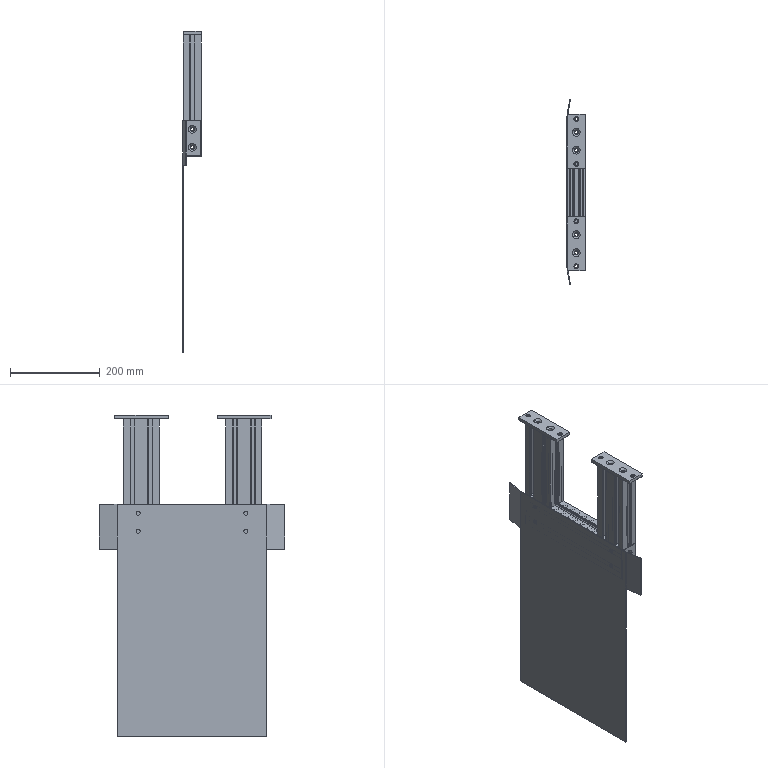Part | SolidWorks | features ReferencePattern 2, LocalLPattern 1 | 8 solids | 1112 faces | box 41.5 x 411.771 x 715 mm | volume 1109076 mm3 | cylinder 558 | plane 538 | cone 16 | commonest cylinder face diameters 0.6 x266 2 x120 0.4 x44 9 x40 6.8 x28 15 x16